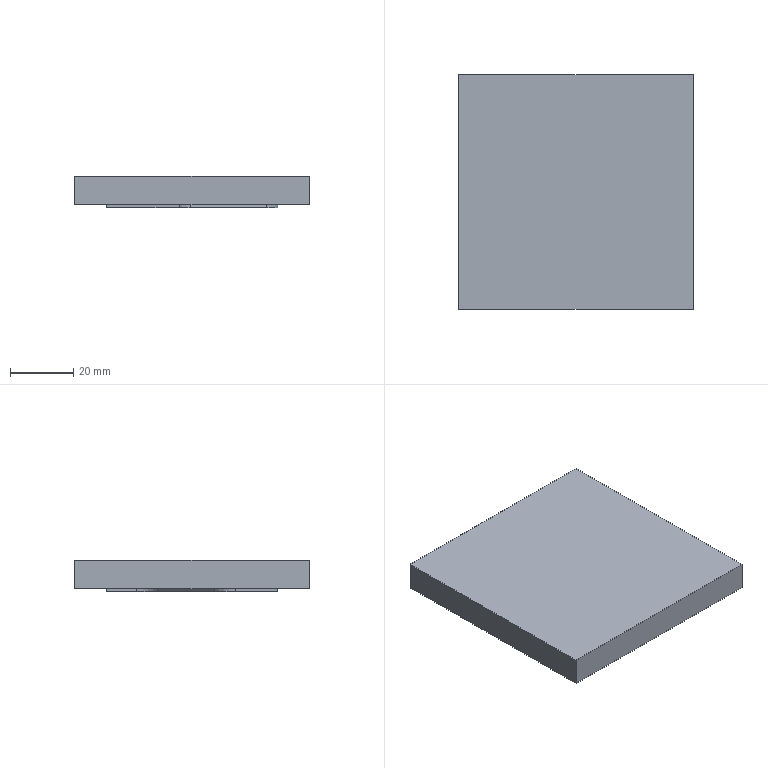NC program | NX | posted with a generic post | part box 74 x 74 x 10 mm
Whole program:
N10 G17 G21 G94 G90
(ZLEVEL_PROFILE_1_COPY_1 , TOOL : D10)
N12 T04 M6
N14 G54
N16 G17 G0 G90 X-22.323 Y33. B0. C0. S7500 M3
N18 G43 Z30. H4
N20 Z6.5
N22 G94 G1 X-27. Z6.255 F1000.
N24 X-27.601 Z6.223
N26 X-29.203 Y32.613 Z6.137
N28 X-30.641 Y31.807 Z6.051
N30 X-31.807 Y30.641 Z5.964
N32 X-32.613 Y29.203 Z5.878
N34 X-33. Y27.601 Z5.791
N36 Y27. Z5.76
N38 Y6.871 Z4.705
N40 Y5.954 Z4.657
N42 X-32.657 Y3.656 Z4.535
N44 X-31.939 Y1.446 Z4.413
N46 X-30.866 Y-0.616 Z4.292
N48 X-29.467 Y-2.472 Z4.17
N50 X-27.781 Y-4.071 Z4.048
N52 X-27.03 Y-4.597 Z4.
N54 X-2.853 Y-21.526 F3000.
N56 G2 X-2. Y-23.165 R2.
N58 G1 Y-27.
N60 G3 X4. Y-33. R6.
N62 G1 X27.
N64 G3 X33. Y-27. R6.
N66 G1 Y-13.665
N68 G3 X27.03 Y-2.196 R14.
N70 G1 X1.353 Y15.783
N72 G2 X0.5 Y17.421 R2.
N74 G1 Y27.
N76 G3 X-5.5 Y33. R6.
N78 G1 X-27.
N80 G3 X-33. Y27. R6.
N82 G1 Y6.871
N84 G3 X-27.03 Y-4.597 R14.
N86 G1 X-26.587 Y-4.907 Z3.991
N88 X-3.123 Y-21.337 Z3.491
N90 X-2.9 Y-21.494 Z3.486
N92 X-2.685 Y-21.658 Z3.481
N94 X-2.495 Y-21.847 Z3.476
N96 X-2.332 Y-22.062 Z3.472
N98 X-2.197 Y-22.298 Z3.467
N100 X-2.098 Y-22.547 Z3.462
N102 X-2.032 Y-22.806 Z3.458
N104 X-2.002 Y-23.077 Z3.453
N106 X-2. Y-23.618 Z3.443
N108 Y-24.158 Z3.434
N110 Y-26.32 Z3.396
N112 Y-26.86 Z3.387
N114 X-1.987 Y-27.401 Z3.377
N116 X-1.926 Y-27.937 Z3.368
N118 X-1.818 Y-28.467 Z3.358
N120 X-1.461 Y-29.486 Z3.34
N122 X-0.927 Y-30.424 Z3.321
N124 X-0.234 Y-31.251 Z3.302
N126 X0.596 Y-31.941 Z3.283
N128 X1.537 Y-32.471 Z3.264
N130 X2.557 Y-32.824 Z3.245
N132 X3.624 Y-32.988 Z3.226
N134 X4.164 Y-33. Z3.217
N136 X4.705 Z3.208
N138 X16.054 Z3.009
N140 X16.595 Z3.
N142 X27.
N144 G3 X33. Y-27. R6.
N146 G1 Y-13.665
N148 G3 X27.03 Y-2.196 R14.
N150 G1 X1.353 Y15.783
N152 G2 X0.5 Y17.421 R2.
N154 G1 Y27.
N156 G3 X-5.5 Y33. R6.
N158 G1 X-27.
N160 G3 X-33. Y27. R6.
N162 G1 Y6.871
N164 G3 X-27.03 Y-4.597 R14.
N166 G1 X-26.587 Y-4.907 Z2.991
N168 X-3.123 Y-21.337 Z2.491
N170 X-2.9 Y-21.494 Z2.486
N172 X-2.685 Y-21.658 Z2.481
N174 X-2.495 Y-21.847 Z2.476
N176 X-2.332 Y-22.062 Z2.472
N178 X-2.197 Y-22.298 Z2.467
N180 X-2.098 Y-22.547 Z2.462
N182 X-2.032 Y-22.806 Z2.458
N184 X-2.002 Y-23.077 Z2.453
N186 X-2. Y-23.618 Z2.443
N188 Y-24.158 Z2.434
N190 Y-26.32 Z2.396
N192 Y-26.86 Z2.387
N194 X-1.987 Y-27.401 Z2.377
N196 X-1.926 Y-27.937 Z2.368
N198 X-1.818 Y-28.467 Z2.358
N200 X-1.461 Y-29.486 Z2.34
N202 X-0.927 Y-30.424 Z2.321
N204 X-0.234 Y-31.251 Z2.302
N206 X0.596 Y-31.941 Z2.283
N208 X1.537 Y-32.471 Z2.264
N210 X2.557 Y-32.824 Z2.245
N212 X3.624 Y-32.988 Z2.226
N214 X4.164 Y-33. Z2.217
N216 X4.705 Z2.208
N218 X16.054 Z2.009
N220 X16.595 Z2.
N222 X27.
N224 G3 X33. Y-27. R6.
N226 G1 Y-13.665
N228 G3 X27.03 Y-2.196 R14.
N230 G1 X1.353 Y15.783
N232 G2 X0.5 Y17.421 R2.
N234 G1 Y27.
N236 G3 X-5.5 Y33. R6.
N238 G1 X-27.
N240 G3 X-33. Y27. R6.
N242 G1 Y6.871
N244 G3 X-27.03 Y-4.597 R14.
N246 G1 X-26.587 Y-4.907 Z1.991
N248 X-3.123 Y-21.337 Z1.491
N250 X-2.9 Y-21.494 Z1.486
N252 X-2.685 Y-21.658 Z1.481
N254 X-2.495 Y-21.847 Z1.476
N256 X-2.332 Y-22.062 Z1.472
N258 X-2.197 Y-22.298 Z1.467
N260 X-2.098 Y-22.547 Z1.462
N262 X-2.032 Y-22.806 Z1.458
N264 X-2.002 Y-23.077 Z1.453
N266 X-2. Y-23.618 Z1.443
N268 Y-24.158 Z1.434
N270 Y-26.32 Z1.396
N272 Y-26.86 Z1.387
N274 X-1.987 Y-27.401 Z1.377
N276 X-1.926 Y-27.937 Z1.368
N278 X-1.818 Y-28.467 Z1.358
N280 X-1.461 Y-29.486 Z1.34
N282 X-0.927 Y-30.424 Z1.321
N284 X-0.234 Y-31.251 Z1.302
N286 X0.596 Y-31.941 Z1.283
N288 X1.537 Y-32.471 Z1.264
N290 X2.557 Y-32.824 Z1.245
N292 X3.624 Y-32.988 Z1.226
N294 X4.164 Y-33. Z1.217
N296 X4.705 Z1.208
N298 X16.054 Z1.009
N300 X16.595 Z1.
N302 X27.
N304 G3 X33. Y-27. R6.
N306 G1 Y-13.665
N308 G3 X27.03 Y-2.196 R14.
N310 G1 X1.353 Y15.783
N312 G2 X0.5 Y17.421 R2.
N314 G1 Y27.
N316 G3 X-5.5 Y33. R6.
N318 G1 X-27.
N320 G3 X-33. Y27. R6.
N322 G1 Y6.871
N324 G3 X-27.03 Y-4.597 R14.
N326 G1 X-26.587 Y-4.907 Z0.991
N328 X-3.123 Y-21.337 Z0.491
N330 X-2.9 Y-21.494 Z0.486
N332 X-2.685 Y-21.658 Z0.481
N334 X-2.495 Y-21.847 Z0.476
N336 X-2.332 Y-22.062 Z0.472
N338 X-2.197 Y-22.298 Z0.467
N340 X-2.098 Y-22.547 Z0.462
N342 X-2.032 Y-22.806 Z0.458
N344 X-2.002 Y-23.077 Z0.453
N346 X-2. Y-23.618 Z0.443
N348 Y-24.158 Z0.434
N350 Y-26.32 Z0.396
N352 Y-26.86 Z0.387
N354 X-1.987 Y-27.401 Z0.377
N356 X-1.926 Y-27.937 Z0.368
N358 X-1.818 Y-28.467 Z0.358
N360 X-1.461 Y-29.486 Z0.34
N362 X-0.927 Y-30.424 Z0.321
N364 X-0.234 Y-31.251 Z0.302
N366 X0.596 Y-31.941 Z0.283
N368 X1.537 Y-32.471 Z0.264
N370 X2.557 Y-32.824 Z0.245
N372 X3.624 Y-32.988 Z0.226
N374 X4.164 Y-33. Z0.217
N376 X4.705 Z0.208
N378 X16.054 Z0.009
N380 X16.595 Z0.
N382 X27.
N384 G3 X33. Y-27. R6.
N386 G1 Y-13.665
N388 G3 X27.03 Y-2.196 R14.
N390 G1 X1.353 Y15.783
N392 G2 X0.5 Y17.421 R2.
N394 G1 Y27.
N396 G3 X-5.5 Y33. R6.
N398 G1 X-27.
N400 G3 X-33. Y27. R6.
N402 G1 Y6.871
N404 G3 X-27.03 Y-4.597 R14.
N406 G1 X-26.587 Y-4.907 Z-0.009
N408 X-3.123 Y-21.337 Z-0.509
N410 X-2.9 Y-21.494 Z-0.514
N412 X-2.685 Y-21.658 Z-0.519
N414 X-2.495 Y-21.847 Z-0.524
N416 X-2.332 Y-22.062 Z-0.528
N418 X-2.197 Y-22.298 Z-0.533
N420 X-2.098 Y-22.547 Z-0.538
N422 X-2.032 Y-22.806 Z-0.542
N424 X-2.002 Y-23.077 Z-0.547
N426 X-2. Y-23.618 Z-0.557
N428 Y-24.158 Z-0.566
N430 Y-26.32 Z-0.604
N432 Y-26.86 Z-0.613
N434 X-1.987 Y-27.401 Z-0.623
N436 X-1.926 Y-27.937 Z-0.632
N438 X-1.818 Y-28.467 Z-0.642
N440 X-1.461 Y-29.486 Z-0.66
N442 X-0.927 Y-30.424 Z-0.679
N444 X-0.234 Y-31.251 Z-0.698
N446 X0.596 Y-31.941 Z-0.717
N448 X1.537 Y-32.471 Z-0.736
N450 X2.557 Y-32.824 Z-0.755
N452 X3.624 Y-32.988 Z-0.774
N454 X4.164 Y-33. Z-0.783
N456 X4.705 Z-0.792
N458 X16.054 Z-0.991
N460 X16.595 Z-1.
N462 X27.
N464 G3 X33. Y-27. R6.
N466 G1 Y-13.665
N468 G3 X27.03 Y-2.196 R14.
N470 G1 X1.353 Y15.783
N472 G2 X0.5 Y17.421 R2.
N474 G1 Y27.
N476 G3 X-5.5 Y33. R6.
N478 G1 X-27.
N480 G3 X-33. Y27. R6.
N482 G1 Y6.871
N484 G3 X-27.03 Y-4.597 R14.
N486 G1 X-2.853 Y-21.526
N488 G2 X-2. Y-23.165 R2.
N490 G1 Y-27.
N492 G3 X4. Y-33. R6.
N494 G1 X16.595
N496 Z0.5
N498 G0 Z30.
N500 M5
(FLOOR_WALL_1_COPY , TOOL : D63)
N502 T03 M6
N504 G54
N506 G17 G0 G90 X-64.5 Y29.997 B0. C0. S6500 M3
N508 G43 Z30. H3
N510 Z7.
N512 G94 G1 Z4. F1500.
N514 X-61.5
N516 X61.5
N518 Y-4.8
N520 X-61.5
N522 X-64.5
N524 Z7.
N526 G0 Z30.
N528 Y29.997
N530 Z6.
N532 G1 Z3.
N534 X-61.5
N536 X61.5
N538 Y-4.8
N540 X-61.5
N542 X-64.5
N544 Z6.
N546 G0 Z30.
N548 Y29.997
N550 Z5.
N552 G1 Z2.
N554 X-61.5
N556 X61.5
N558 Y-4.8
N560 X-61.5
N562 X-64.5
N564 Z5.
N566 G0 Z30.
N568 Y29.997
N570 Z4.
N572 G1 Z1.
N574 X-61.5
N576 X61.5
N578 Y-4.8
N580 X-61.5
N582 X-64.5
N584 Z4.
N586 G0 Z30.
N588 Y29.997
N590 Z3.
N592 G1 Z0.
N594 X-61.5
N596 X61.5
N598 Y-4.8
N600 X-61.5
N602 X-64.5
N604 Z3.
N606 G0 Z30.
N608 M5
N610 M2